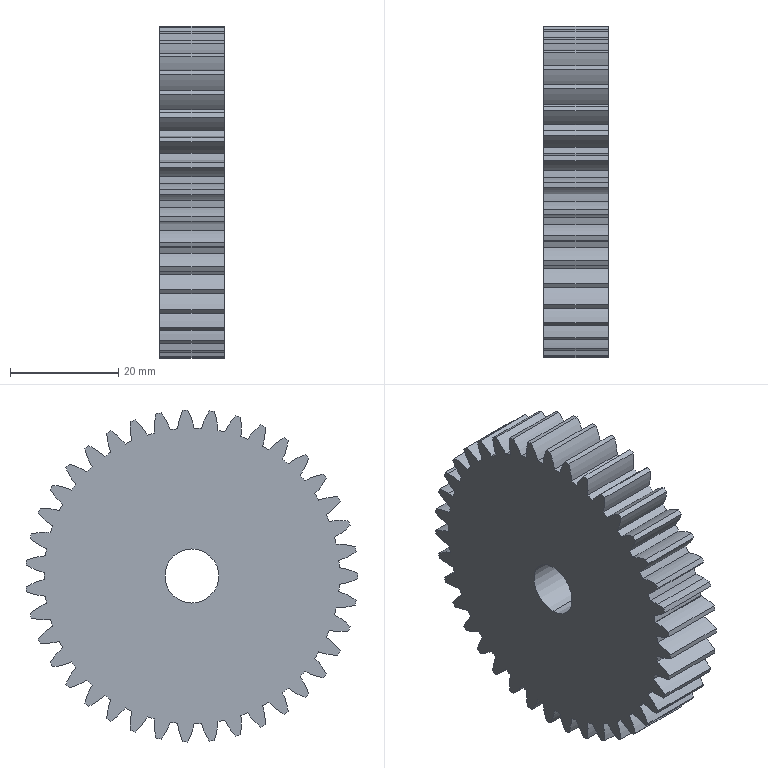Part | SolidWorks | features Boss 3, Cut 3, CirPattern 2, Fillet 2, Revolution 1 | 1 solid | 164 faces | box 12 x 61.434 x 61.481 mm | volume 30777 mm3 | cylinder 162 | plane 2 | commonest cylinder face diameters 23.4 x82 54.748 x39 61.5 x39 10 x2